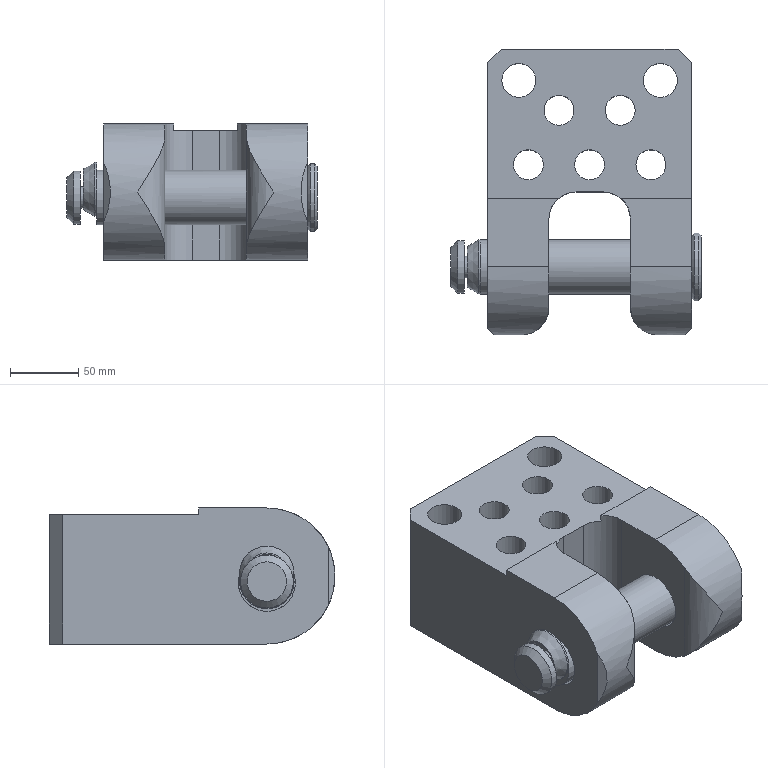Part | NX | features solid 2 | 1 solid | 261 faces | box 184 x 210 x 100 mm | volume 2117803 mm3 | plane 127 | spline 104 | cylinder 26 | cone 4 | commonest cylinder face diameters 40 x6 22 x5 33 x5 25 x2 42 x2 100 x2